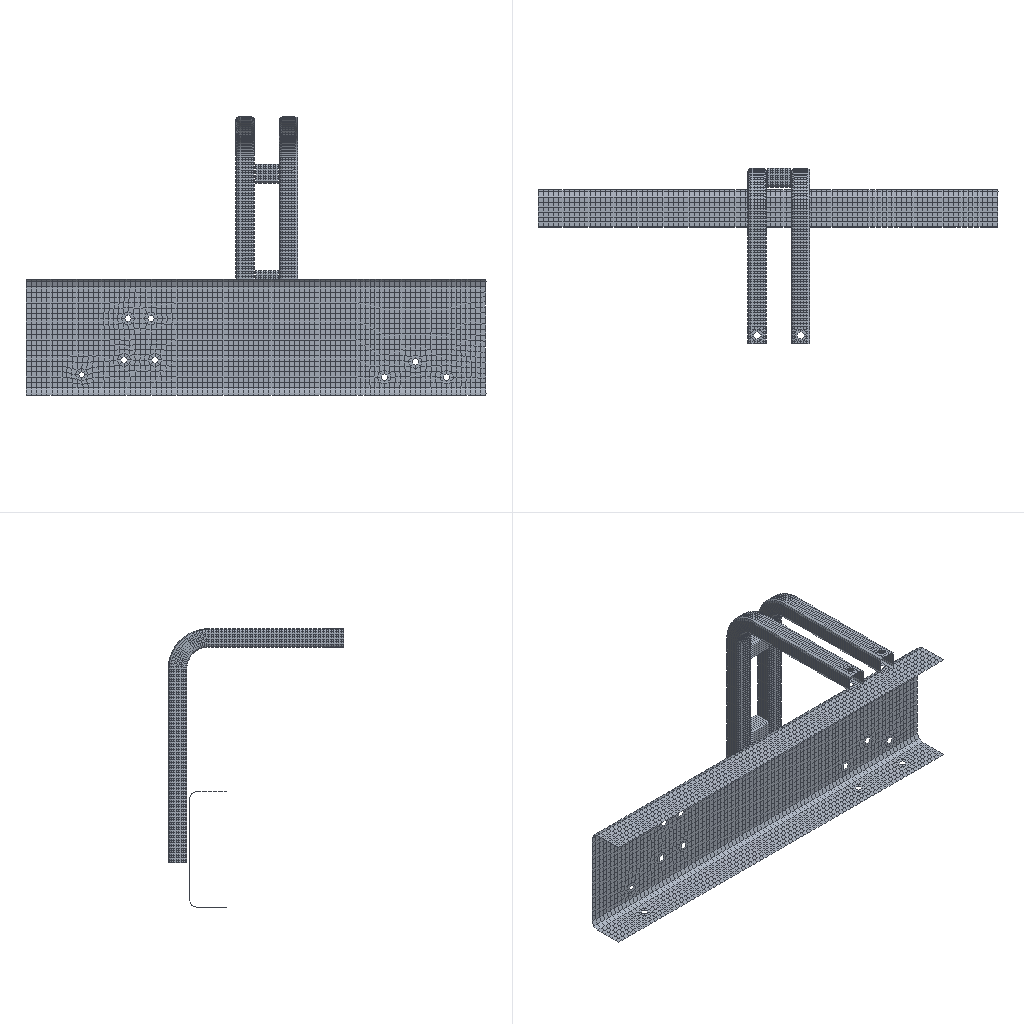Simulation study | nastran
Set-up summary:
category,name,step,type,value,unit,region
solver,nx_nastran
units,not stated in the deck,,not stated
analysis,deck,,static,static
analysis,solution,,SOL,101
load_step,SUBCASE 1,1,SUBCASE,SPC=6 LOAD=1
load_step,SUBCASE 2,2,SUBCASE,SPC=6 LOAD=2
load_step,SUBCASE 3,3,SUBCASE,SPC=6 LOAD=3
load_step,SUBCASE 4,4,SUBCASE,SPC=6 LOAD=4
load_step,requested,,,4
mesh,nodes,,,11798
mesh,elements,,,11479
element_type,CONM2,,mass,1
element_type,CQUAD4,,shell,11430
element_type,CTRIA3,,shell,48
load,load commands in deck,,count,4
bc,support commands in deck,,count,72
check,setup vs results,,match,"every grid point's frame and coordinates and every element id; grid points of CQUAD4, CTRIA3 elements"
Nastran input file, long lists of numbers shortened:
$$------------------------------------------------------------------------------$
$$                                                                              $
$$ NASTRAN Input Deck Generated by HyperMesh Version  : 9.0b121                 $
$$ Generated using HyperMesh-Nastran Template Version : 9.0b121
$$                                                                              $
$$   Template:  general                                                         $
$$                                                                              $
$$------------------------------------------------------------------------------$
$$------------------------------------------------------------------------------$
$$                      Executive Control Cards                                 $
$$------------------------------------------------------------------------------$
SOL 101
CEND
$$------------------------------------------------------------------------------$
$$                      Case Control Cards                                      $
$$------------------------------------------------------------------------------$
  DISPLACEMENT(PLOT) = ALL
  STRESS(PLOT) = ALL
  STRAIN(PLOT) = ALL
$
$HMNAME LOADSTEP               1"Step_X2g"
SUBCASE       1
  LABEL=      Step_X2g
  SPC =        6
  LOAD =        1
$
$HMNAME LOADSTEP               2"Step_Y2g"
SUBCASE       2
  LABEL=      Step_Y2g
  SPC =        6
  LOAD =        2
$
$HMNAME LOADSTEP               3"Step_Z2g"
SUBCASE       3
  LABEL=      Step_Z2g
  SPC =        6
  LOAD =        3
$
$HMNAME LOADSTEP               4"Step_Z-4g"
SUBCASE       4
  LABEL=      Step_Z-4g
  SPC =        6
  LOAD =        4
$$------------------------------------------------------------------------------$
$$                      Bulk Data Cards                                         $
$$------------------------------------------------------------------------------$
BEGIN BULK
PARAM,BAILOUT,-1
PARAM,POST,-1
$$
$$  GRID Data
$$
GRID          71        388.0   434.4997233.4314
GRID          72        388.0   434.5   228.4144
$ (11796 more lines like these left out)
$$
$$  SPOINT Data
$$
$
$  CONM2 Elements
$
CONM2     176473  207939       00.0065  0.0     0.0     0.0
$
$HMMOVE  2801015
$         176473
$
$$
$$------------------------------------------------------------------------------$
$$             Group Definitions                                                $
$$------------------------------------------------------------------------------$
$
$ RBE2 Elements - Single dependent node
$
RBE2      176416  207678  123456    6257
RBE2      176417  207703  123456    6274
$ (54 more lines like these left out)
$
$HMMOVE       13
$         176416THRU      176471
$
$$
$$ RBE2 Elements - Multiple dependent nodes
$$
RBE2      176472  207939  123456    2818    2830    2841    2855    2856+
+           2871    3109    3110    3111    3112    3113    3204    3205+
+           3206    3207    3208    3209    3210    3211    3375    3378+
+           3379    3381    3382    3383    3384    3385    3386    3387+
+           3388    3389    6766    6770    6772    6781    6783    6784+
+           6785    6786    6787    6792    6793    6794    6795    6813+
+           6814    6815    6817    6819    6820    6821    6822    6824+
+           6825    6833    6834    6835    6836    7174  205063  205064+
+         205065  205066  205067  205068  205069  205070  205071  205072+
+         205073  205074  205075  205076  205077  205078  205079  205080+
+         205081  205082  205083  205084  205085  205089  205090  205091+
+         205092  205093  205094  205095  205096  205097  205098  205099+
+         205100  205101  205102  205103  205104  205105  205106  205107+
+         205108  205109  205110  205111  205112  205120  205121  205122+
+         205867  205868  205869  205874  205875  205876  205878  205879+
+         205880  205881  205882  205883  205884  205885  205886  205887+
+         205888  205889  205890  205891  205892  205893  205894  205895+
+         205896  205897  205898  205899  205900  206095  206096  206097+
+         206098  206099  206190  206191  206192  206193  206194  206195+
+         206196  206310  206313  206314  206316  206317  206318  206319+
+         206320  206321  206322  206323  206324
RBE2      176475  207941  123456  185505  185506  185523  185526  204162+
+         204163  204164  204165  204166  204167  204168  204169  204170+
+         204171  204172  204173  204174  204175  204176  204177  204178+
+         204179  204180  204181  204182  204183  204184  204185  204186+
+         204187  204188  204189  204195  204196  204197  204198  204199+
+         204200  204201  204202  204203  204204  204205  204206  204207+
+         204208  204209  204210  204211  204212  204213  204214  204215+
+         204216  204217  204218  204219  204220  204221  204222
RBE2      176476  207942  123456  185455  185456  185641  185662  204134+
+         204135  204136  204137  204138  204139  204140  204141  204142+
+         204143  204144  204145  204146  204147  204148  204149  204150+
+         204151  204152  204153  204154  204155  204156  204157  204158+
+         204159  204160  204161  204223  204224  204225  204226  204227+
+         204228  204229  204230  204231  204232  204233  204234  204235+
+         204236  204237  204238  204239  204240  204241  204242  204243+
+         204244  204245  204246  204247  204248  204249  204250
RBE2      176477  207943  123456    5201    5202    5203    5204    5205+
+           5206    5207    5208    5209    5210    5211    5212    5213+
+           5214    5215    5216    5217    5218    5219    5220    5221+
+           5222    5223    5224    5225    5226    5227    5228    5234+
+           5235    5236    5237    5238    5239    5240    5241    5242+
+           5243    5244    5245    5246    5247    5248    5249    5250+
+           5251    5252    5253    5254    5255    5256    5257    5258+
+           5259    5260    5261  185862  185863  185881  185885
RBE2      176478  207944  123456    5173    5174    5175    5176    5177+
+           5178    5179    5180    5181    5182    5183    5184    5185+
+           5186    5187    5188    5189    5190    5191    5192    5193+
+           5194    5195    5196    5197    5198    5199    5200    5262+
+           5263    5264    5265    5266    5267    5268    5269    5270+
+           5271    5272    5273    5274    5275    5276    5277    5278+
+           5279    5280    5281    5282    5283    5284    5285    5286+
+           5287    5288    5289  185753  185754  186015  186038
$
$HMMOVE       13
$         176472  176475THRU      176478
$
$$
$$  CTRIA3 Data
$$
CTRIA3      4593       1  204013  204014  204015
CTRIA3      4633       1  204190  204093    1102
$ (46 more lines like these left out)
$
$HMMOVE       11
$           4593    4633    4606    4600    4567    4595    4558    4622    4611
$           4583    4616    4578    4627    4507    4492    4550    4485    4501
$           4562    4468    4572    4493    4478    4464    5031    5134    5160
$           5162    5287    5320    5348    5457  174248    5486    5509    5826
$           5985  174523  174526  174528  174557  174591  174692    7105  174983
$         175081  175907THRU      175908
$
$
$  CQUAD4 Elements
$
CQUAD4    172175       2  184132  198397  203057  184134
CQUAD4    172176       2  184099  184036  198397  184132
$ (11428 more lines like these left out)
$
$HMMOVE  2801014
$         172175THRU      172180  168238THRU      168239  166874  166881THRU
$         166882  166890  166898  166902  162744THRU      162761  160572THRU
$ (287 more lines like these left out)
PSHELL         2       16.0            1               1
$
$HMNAME PROP                   1"Pshell_400T" 4
$HWCOLOR PROP                  1      11
PSHELL         1       14.0            1               1
$$
$$------------------------------------------------------------------------------$
$$                      Material Definition Cards                               $
$$------------------------------------------------------------------------------$
$$--------------------------------------------------------------
$$ HYPERMESH TAGS
$$--------------------------------------------------------------
$$BEGIN TAGS
$$END TAGS
$$
$$  MAT1 Data
$
$HMNAME MAT                    1"Steel" "MAT1"
$HWCOLOR MAT                   1      11
MAT1           1210000.0        0.3     7.90E-09
$$
$$
$$
$$------------------------------------------------------------------------------$
$ (27 more lines like these left out)
GRAV           1        9800.0  2.0     0.0     0.0
$$
$HMNAME LOADCOL                2"Y2g"
$HWCOLOR LOADCOL               2       4
GRAV           2        9800.0  0.0     2.0     0.0
$$
$HMNAME LOADCOL                3"Z2g"
$HWCOLOR LOADCOL               3       5
GRAV           3        9800.0  0.0     0.0     2.0
$$
$HMNAME LOADCOL                4"Z-4g"
$HWCOLOR LOADCOL               4       6
GRAV           4        9800.0  0.0     0.0     -4.0
$$
$$
$$
$$
$$
$$
$$
$$
$$
$$
$$
$$  SPC Data
$$
SPC            6  172412  1234560.0
SPC            6  172429  1234560.0
SPC            6  173106  1234560.0
SPC            6  174844  1234560.0
$ (68 more lines like these left out)
$HMASSEM   28010       3 2801
$HMASSEM_IDS     2801014
$
ENDDATA
Results summary:
result,analysis,,,static
result,last_loadstep,,,4
result,primary field,,,displacements
result,max displacement,,,0.4976,model units